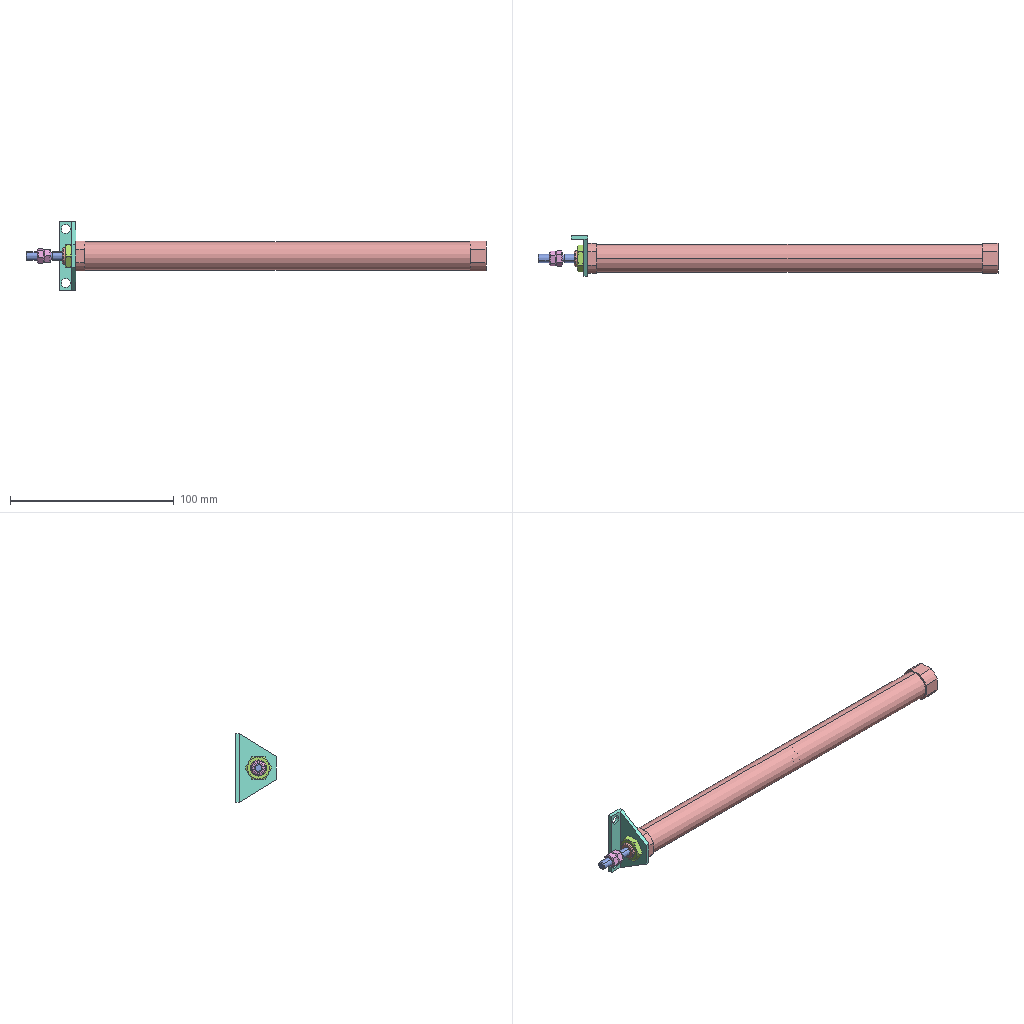Assembly | SolidWorks | 5 different items | 6 placed | box 281 x 25 x 42 mm
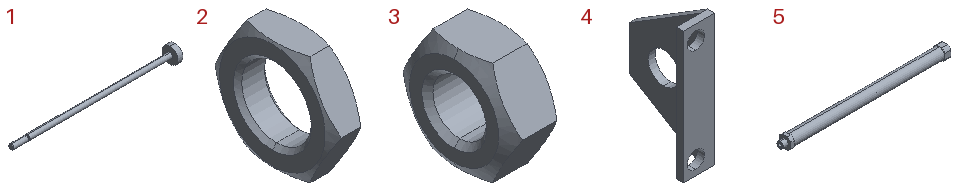Parts list (item | quantity | size | volume | features):
1 | x1 | 163.5 x 16 x 16 mm | 4106 mm3 | features Revolution 1
2 | x1 | 4 x 16.166 x 14 mm | 408.53 mm3 | features BaseBody 1
3 | x2 | 4 x 9.238 x 8 mm | 156.613 mm3 | features BaseBody 1
4 | x1 | 10 x 25 x 42 mm | 2138 mm3 | features HoleWzd 2, Chamfer 1, Extrusion 1, ICE 1
5 | x1 | 259 x 18.3 x 18.3 mm | 34694 mm3 | features Chamfer 2, HoleWzd 2, ICE 2, Extrusion 1, Revolution 1
Mates (type | each side: item.copy, entity, surface, feature):
Concentric | 5.1 face cylinder CBORE for M13 SHSS1 | 1.1 face cylinder Revolve1
Concentric | 5.1 face cylinder Revolve1 | 4.1 face cylinder Ø10.0 (10) Diameter Hole1
Coincident | 5.1 face plane Boss-Extrude1 | 4.1 face plane Boss-Extrude1
Parallel | 5.1 face plane Boss-Extrude1 | 4.1 face plane Boss-Extrude1
Coincident | 2.1 face plane Input1 | 4.1 face plane Boss-Extrude1
Coincident | 1.1 face plane Revolve1 | 3.1 face plane Input1
Coincident | 3.1 face plane Input1 | 3.2 face plane Input1
LimitDistanceDim | 1.1 face plane Revolve1 | 4.1 face plane Boss-Extrude1
Concentric | 1.1 face cylinder Revolve1 | 3.2 face cylinder Input1
Concentric | 5.1 face cylinder Revolve1 | 2.1 face cylinder Input1
Concentric | 1.1 face cylinder Revolve1 | 3.1 face cylinder Input1